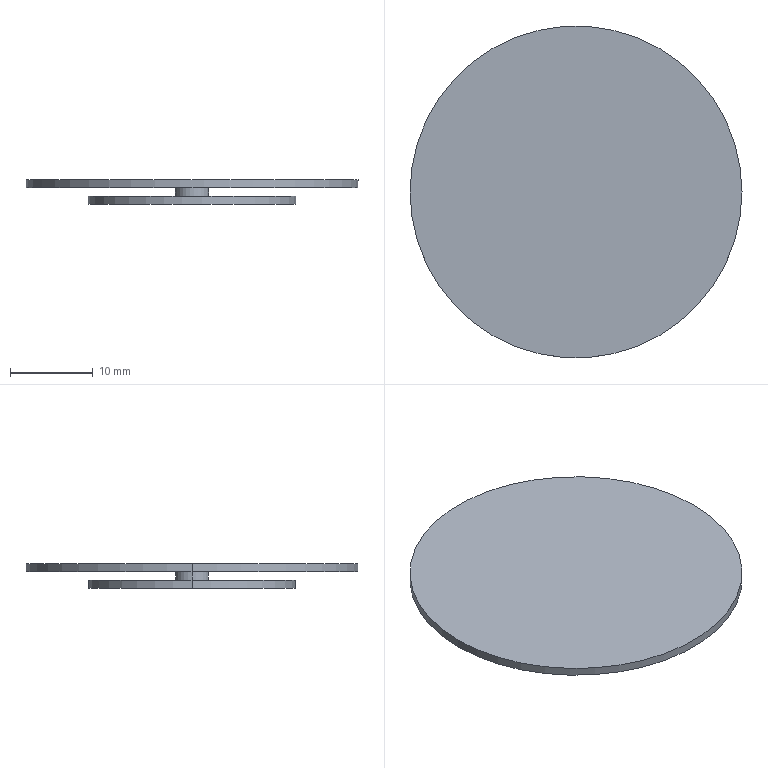Part | SolidWorks | features ICE 2, Extrusion 1 | 1 solid | 10 faces | box 40 x 40 x 3 mm | volume 1760 mm3 | cylinder 6 | plane 4 | commonest cylinder face diameters 4 x2 25 x2 40 x2
STEP:
#1=CARTESIAN_POINT('',(-12.5,0.,-2.));
#2=VERTEX_POINT('',#1);
#3=CARTESIAN_POINT('',(12.5,0.,-2.));
#4=VERTEX_POINT('',#3);
#5=CARTESIAN_POINT('',(0.,0.,-2.));
#6=DIRECTION('',(0.,0.,-1.));
#7=DIRECTION('',(-1.,0.,0.));
#8=AXIS2_PLACEMENT_3D('',#5,#6,#7);
#9=CIRCLE('',#8,12.5);
#10=EDGE_CURVE('',#2,#4,#9,.T.);
#11=ORIENTED_EDGE('',*,*,#10,.F.);
#12=CARTESIAN_POINT('',(-12.5,0.,-1.));
#13=VERTEX_POINT('',#12);
#14=CARTESIAN_POINT('',(-12.5,0.,-2.));
#15=DIRECTION('',(0.,0.,1.));
#16=VECTOR('',#15,1000.);
#17=LINE('',#14,#16);
#18=EDGE_CURVE('',#2,#13,#17,.T.);
#19=ORIENTED_EDGE('',*,*,#18,.T.);
#20=CARTESIAN_POINT('',(12.5,0.,-1.));
#21=VERTEX_POINT('',#20);
#22=CARTESIAN_POINT('',(0.,0.,-1.));
#23=DIRECTION('',(0.,0.,-1.));
#24=DIRECTION('',(-1.,0.,0.));
#25=AXIS2_PLACEMENT_3D('',#22,#23,#24);
#26=CIRCLE('',#25,12.5);
#27=EDGE_CURVE('',#13,#21,#26,.T.);
#28=ORIENTED_EDGE('',*,*,#27,.T.);
#29=CARTESIAN_POINT('',(12.5,0.,-2.));
#30=DIRECTION('',(0.,0.,1.));
#31=VECTOR('',#30,1000.);
#32=LINE('',#29,#31);
#33=EDGE_CURVE('',#4,#21,#32,.T.);
#34=ORIENTED_EDGE('',*,*,#33,.F.);
#35=EDGE_LOOP('',(#11,#19,#28,#34));
#36=FACE_OUTER_BOUND('',#35,.T.);
#37=CARTESIAN_POINT('',(0.,0.,-2.));
#38=DIRECTION('',(0.,0.,1.));
#39=DIRECTION('',(1.,0.,0.));
#40=AXIS2_PLACEMENT_3D('',#37,#38,#39);
#41=CYLINDRICAL_SURFACE('',#40,12.5);
#42=ADVANCED_FACE('',(#36),#41,.T.);
#43=CARTESIAN_POINT('',(-2.,0.,-1.));
#44=VERTEX_POINT('',#43);
#45=CARTESIAN_POINT('',(2.,0.,-1.));
#46=VERTEX_POINT('',#45);
#47=CARTESIAN_POINT('',(0.,0.,-1.));
#48=DIRECTION('',(0.,0.,-1.));
#49=DIRECTION('',(-1.,0.,0.));
#50=AXIS2_PLACEMENT_3D('',#47,#48,#49);
#51=CIRCLE('',#50,2.);
#52=EDGE_CURVE('',#44,#46,#51,.T.);
#53=ORIENTED_EDGE('',*,*,#52,.F.);
#54=CARTESIAN_POINT('',(-2.,0.,0.));
#55=VERTEX_POINT('',#54);
#56=CARTESIAN_POINT('',(-2.,0.,-1.));
#57=DIRECTION('',(0.,0.,1.));
#58=VECTOR('',#57,1000.);
#59=LINE('',#56,#58);
#60=EDGE_CURVE('',#44,#55,#59,.T.);
#61=ORIENTED_EDGE('',*,*,#60,.T.);
#62=CARTESIAN_POINT('',(2.,0.,0.));
#63=VERTEX_POINT('',#62);
#64=CARTESIAN_POINT('',(0.,0.,0.));
#65=DIRECTION('',(0.,0.,-1.));
#66=DIRECTION('',(1.,0.,0.));
#67=AXIS2_PLACEMENT_3D('',#64,#65,#66);
#68=CIRCLE('',#67,2.);
#69=EDGE_CURVE('',#55,#63,#68,.T.);
#70=ORIENTED_EDGE('',*,*,#69,.T.);
#71=CARTESIAN_POINT('',(2.,0.,-1.));
#72=DIRECTION('',(0.,0.,1.));
#73=VECTOR('',#72,1000.);
#74=LINE('',#71,#73);
#75=EDGE_CURVE('',#46,#63,#74,.T.);
#76=ORIENTED_EDGE('',*,*,#75,.F.);
#77=EDGE_LOOP('',(#53,#61,#70,#76));
#78=FACE_OUTER_BOUND('',#77,.T.);
#79=CARTESIAN_POINT('',(0.,0.,-1.));
#80=DIRECTION('',(0.,0.,1.));
#81=DIRECTION('',(1.,0.,0.));
#82=AXIS2_PLACEMENT_3D('',#79,#80,#81);
#83=CYLINDRICAL_SURFACE('',#82,2.);
#84=ADVANCED_FACE('',(#78),#83,.T.);
#85=CARTESIAN_POINT('',(20.,0.,1.));
#86=VERTEX_POINT('',#85);
#87=CARTESIAN_POINT('',(-20.,0.,1.));
#88=VERTEX_POINT('',#87);
#89=CARTESIAN_POINT('',(0.,0.,1.));
#90=DIRECTION('',(0.,0.,1.));
#91=DIRECTION('',(1.,0.,0.));
#92=AXIS2_PLACEMENT_3D('',#89,#90,#91);
#93=CIRCLE('',#92,20.);
#94=EDGE_CURVE('',#86,#88,#93,.T.);
#95=ORIENTED_EDGE('',*,*,#94,.F.);
#96=CARTESIAN_POINT('',(20.,0.,0.));
#97=VERTEX_POINT('',#96);
#98=CARTESIAN_POINT('',(20.,0.,1.));
#99=DIRECTION('',(0.,0.,-1.));
#100=VECTOR('',#99,1000.);
#101=LINE('',#98,#100);
#102=EDGE_CURVE('',#86,#97,#101,.T.);
#103=ORIENTED_EDGE('',*,*,#102,.T.);
#104=CARTESIAN_POINT('',(-20.,0.,0.));
#105=VERTEX_POINT('',#104);
#106=CARTESIAN_POINT('',(0.,0.,0.));
#107=DIRECTION('',(0.,0.,1.));
#108=DIRECTION('',(1.,0.,0.));
#109=AXIS2_PLACEMENT_3D('',#106,#107,#108);
#110=CIRCLE('',#109,20.);
#111=EDGE_CURVE('',#97,#105,#110,.T.);
#112=ORIENTED_EDGE('',*,*,#111,.T.);
#113=CARTESIAN_POINT('',(-20.,0.,1.));
#114=DIRECTION('',(0.,0.,-1.));
#115=VECTOR('',#114,1000.);
#116=LINE('',#113,#115);
#117=EDGE_CURVE('',#88,#105,#116,.T.);
#118=ORIENTED_EDGE('',*,*,#117,.F.);
#119=EDGE_LOOP('',(#95,#103,#112,#118));
#120=FACE_OUTER_BOUND('',#119,.T.);
#121=CARTESIAN_POINT('',(0.,0.,1.));
#122=DIRECTION('',(0.,0.,-1.));
#123=DIRECTION('',(-1.,0.,0.));
#124=AXIS2_PLACEMENT_3D('',#121,#122,#123);
#125=CYLINDRICAL_SURFACE('',#124,20.);
#126=ADVANCED_FACE('',(#120),#125,.T.);
#127=ORIENTED_EDGE('',*,*,#102,.F.);
#128=CARTESIAN_POINT('',(0.,0.,1.));
#129=DIRECTION('',(0.,0.,1.));
#130=DIRECTION('',(1.,0.,0.));
#131=AXIS2_PLACEMENT_3D('',#128,#129,#130);
#132=CIRCLE('',#131,20.);
#133=EDGE_CURVE('',#88,#86,#132,.T.);
#134=ORIENTED_EDGE('',*,*,#133,.F.);
#135=ORIENTED_EDGE('',*,*,#117,.T.);
#136=CARTESIAN_POINT('',(0.,0.,0.));
#137=DIRECTION('',(0.,0.,1.));
#138=DIRECTION('',(1.,0.,0.));
#139=AXIS2_PLACEMENT_3D('',#136,#137,#138);
#140=CIRCLE('',#139,20.);
#141=EDGE_CURVE('',#105,#97,#140,.T.);
#142=ORIENTED_EDGE('',*,*,#141,.T.);
#143=EDGE_LOOP('',(#127,#134,#135,#142));
#144=FACE_OUTER_BOUND('',#143,.T.);
#145=CARTESIAN_POINT('',(0.,0.,1.));
#146=DIRECTION('',(0.,0.,-1.));
#147=DIRECTION('',(-1.,0.,0.));
#148=AXIS2_PLACEMENT_3D('',#145,#146,#147);
#149=CYLINDRICAL_SURFACE('',#148,20.);
#150=ADVANCED_FACE('',(#144),#149,.T.);
#151=ORIENTED_EDGE('',*,*,#133,.T.);
#152=ORIENTED_EDGE('',*,*,#94,.T.);
#153=EDGE_LOOP('',(#151,#152));
#154=FACE_OUTER_BOUND('',#153,.T.);
#155=CARTESIAN_POINT('',(0.,0.,1.));
#156=DIRECTION('',(0.,0.,1.));
#157=DIRECTION('',(1.,0.,0.));
#158=AXIS2_PLACEMENT_3D('',#155,#156,#157);
#159=PLANE('',#158);
#160=ADVANCED_FACE('',(#154),#159,.T.);
#161=CARTESIAN_POINT('',(0.,0.,0.));
#162=DIRECTION('',(0.,0.,-1.));
#163=DIRECTION('',(1.,0.,0.));
#164=AXIS2_PLACEMENT_3D('',#161,#162,#163);
#165=CIRCLE('',#164,2.);
#166=EDGE_CURVE('',#63,#55,#165,.T.);
#167=ORIENTED_EDGE('',*,*,#166,.F.);
#168=ORIENTED_EDGE('',*,*,#69,.F.);
#169=EDGE_LOOP('',(#167,#168));
#170=FACE_BOUND('',#169,.T.);
#171=ORIENTED_EDGE('',*,*,#141,.F.);
#172=ORIENTED_EDGE('',*,*,#111,.F.);
#173=EDGE_LOOP('',(#171,#172));
#174=FACE_OUTER_BOUND('',#173,.T.);
#175=CARTESIAN_POINT('',(0.,0.,0.));
#176=DIRECTION('',(0.,0.,1.));
#177=DIRECTION('',(1.,0.,0.));
#178=AXIS2_PLACEMENT_3D('',#175,#176,#177);
#179=PLANE('',#178);
#180=ADVANCED_FACE('',(#170,#174),#179,.F.);
#181=ORIENTED_EDGE('',*,*,#60,.F.);
#182=CARTESIAN_POINT('',(0.,0.,-1.));
#183=DIRECTION('',(0.,0.,-1.));
#184=DIRECTION('',(-1.,0.,0.));
#185=AXIS2_PLACEMENT_3D('',#182,#183,#184);
#186=CIRCLE('',#185,2.);
#187=EDGE_CURVE('',#46,#44,#186,.T.);
#188=ORIENTED_EDGE('',*,*,#187,.F.);
#189=ORIENTED_EDGE('',*,*,#75,.T.);
#190=ORIENTED_EDGE('',*,*,#166,.T.);
#191=EDGE_LOOP('',(#181,#188,#189,#190));
#192=FACE_OUTER_BOUND('',#191,.T.);
#193=CARTESIAN_POINT('',(0.,0.,-1.));
#194=DIRECTION('',(0.,0.,1.));
#195=DIRECTION('',(1.,0.,0.));
#196=AXIS2_PLACEMENT_3D('',#193,#194,#195);
#197=CYLINDRICAL_SURFACE('',#196,2.);
#198=ADVANCED_FACE('',(#192),#197,.T.);
#199=ORIENTED_EDGE('',*,*,#18,.F.);
#200=CARTESIAN_POINT('',(0.,0.,-2.));
#201=DIRECTION('',(0.,0.,-1.));
#202=DIRECTION('',(-1.,0.,0.));
#203=AXIS2_PLACEMENT_3D('',#200,#201,#202);
#204=CIRCLE('',#203,12.5);
#205=EDGE_CURVE('',#4,#2,#204,.T.);
#206=ORIENTED_EDGE('',*,*,#205,.F.);
#207=ORIENTED_EDGE('',*,*,#33,.T.);
#208=CARTESIAN_POINT('',(0.,0.,-1.));
#209=DIRECTION('',(0.,0.,-1.));
#210=DIRECTION('',(-1.,0.,0.));
#211=AXIS2_PLACEMENT_3D('',#208,#209,#210);
#212=CIRCLE('',#211,12.5);
#213=EDGE_CURVE('',#21,#13,#212,.T.);
#214=ORIENTED_EDGE('',*,*,#213,.T.);
#215=EDGE_LOOP('',(#199,#206,#207,#214));
#216=FACE_OUTER_BOUND('',#215,.T.);
#217=CARTESIAN_POINT('',(0.,0.,-2.));
#218=DIRECTION('',(0.,0.,1.));
#219=DIRECTION('',(1.,0.,0.));
#220=AXIS2_PLACEMENT_3D('',#217,#218,#219);
#221=CYLINDRICAL_SURFACE('',#220,12.5);
#222=ADVANCED_FACE('',(#216),#221,.T.);
#223=ORIENTED_EDGE('',*,*,#205,.T.);
#224=ORIENTED_EDGE('',*,*,#10,.T.);
#225=EDGE_LOOP('',(#223,#224));
#226=FACE_OUTER_BOUND('',#225,.T.);
#227=CARTESIAN_POINT('',(0.,0.,-2.));
#228=DIRECTION('',(0.,0.,-1.));
#229=DIRECTION('',(-1.,0.,0.));
#230=AXIS2_PLACEMENT_3D('',#227,#228,#229);
#231=PLANE('',#230);
#232=ADVANCED_FACE('',(#226),#231,.T.);
#233=ORIENTED_EDGE('',*,*,#187,.T.);
#234=ORIENTED_EDGE('',*,*,#52,.T.);
#235=EDGE_LOOP('',(#233,#234));
#236=FACE_BOUND('',#235,.T.);
#237=ORIENTED_EDGE('',*,*,#213,.F.);
#238=ORIENTED_EDGE('',*,*,#27,.F.);
#239=EDGE_LOOP('',(#237,#238));
#240=FACE_OUTER_BOUND('',#239,.T.);
#241=CARTESIAN_POINT('',(0.,0.,-1.));
#242=DIRECTION('',(0.,0.,-1.));
#243=DIRECTION('',(-1.,0.,0.));
#244=AXIS2_PLACEMENT_3D('',#241,#242,#243);
#245=PLANE('',#244);
#246=ADVANCED_FACE('',(#236,#240),#245,.F.);
#247=CLOSED_SHELL('',(#42,#84,#126,#150,#160,#180,#198,#222,#232,#246));
#248=MANIFOLD_SOLID_BREP('',#247);
#249=CARTESIAN_POINT('',(0.,0.,0.));
#250=DIRECTION('',(0.,0.,1.));
#251=DIRECTION('',(1.,0.,0.));
#252=AXIS2_PLACEMENT_3D('',#249,#250,#251);
#253=(LENGTH_UNIT()NAMED_UNIT(*)SI_UNIT(.MILLI.,.METRE.));
#254=UNCERTAINTY_MEASURE_WITH_UNIT(LENGTH_MEASURE(0.00001),#253,'','');
#255=(NAMED_UNIT(*)PLANE_ANGLE_UNIT()SI_UNIT($,.RADIAN.));
#256=(NAMED_UNIT(*)SI_UNIT($,.STERADIAN.)SOLID_ANGLE_UNIT());
#257=(GEOMETRIC_REPRESENTATION_CONTEXT(3)GLOBAL_UNCERTAINTY_ASSIGNED_CONTEXT((#254))GLOBAL_UNIT_ASSIGNED_CONTEXT((#253,#255,#256))REPRESENTATION_CONTEXT('',''));
#258=ADVANCED_BREP_SHAPE_REPRESENTATION('',(#248,#252),#257);